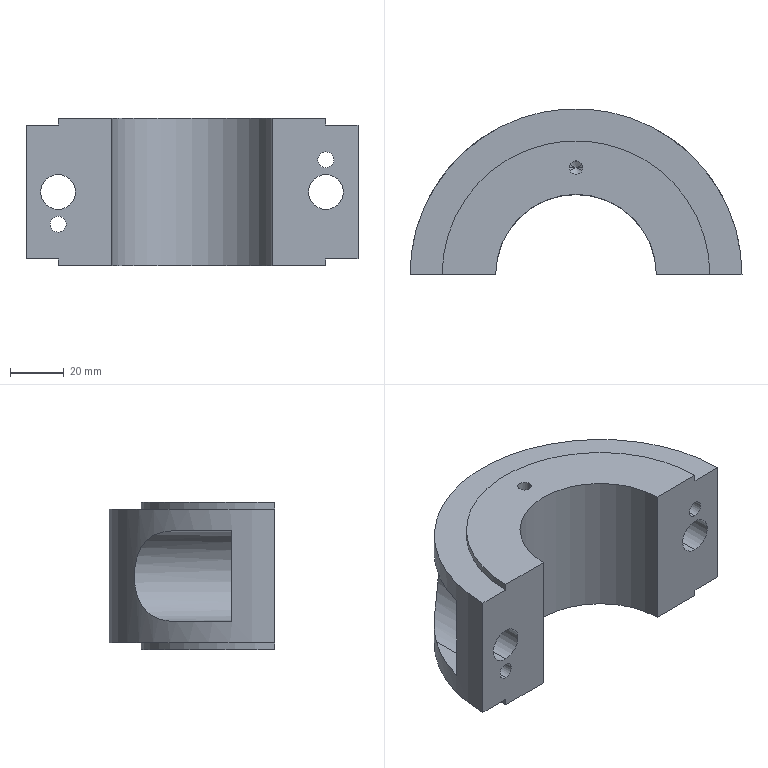Part | SolidWorks | features ICE 3, Extrusion 1, HoleWzd 1 | 1 solid | 30 faces | box 124 x 62 x 55 mm | volume 204402 mm3 | cylinder 16 | plane 12 | cone 2 | commonest cylinder face diameters 6 x4 13 x4 5 x2 34 x2 100 x2 60 x1
STEP:
#1=CARTESIAN_POINT('',(-2.5,40.,10.5));
#2=VERTEX_POINT('',#1);
#3=CARTESIAN_POINT('',(2.5,40.,10.5));
#4=VERTEX_POINT('',#3);
#5=CARTESIAN_POINT('',(0.,40.,10.5));
#6=DIRECTION('',(0.,0.,1.));
#7=DIRECTION('',(1.,0.,0.));
#8=AXIS2_PLACEMENT_3D('',#5,#6,#7);
#9=CIRCLE('',#8,2.5);
#10=EDGE_CURVE('',#2,#4,#9,.T.);
#11=ORIENTED_EDGE('',*,*,#10,.F.);
#12=CARTESIAN_POINT('',(-2.5,40.,27.5));
#13=VERTEX_POINT('',#12);
#14=CARTESIAN_POINT('',(-2.5,40.,27.5));
#15=DIRECTION('',(0.,0.,1.));
#16=VECTOR('',#15,1000.);
#17=LINE('',#14,#16);
#18=EDGE_CURVE('',#2,#13,#17,.T.);
#19=ORIENTED_EDGE('',*,*,#18,.T.);
#20=CARTESIAN_POINT('',(2.5,40.,27.5));
#21=VERTEX_POINT('',#20);
#22=CARTESIAN_POINT('',(0.,40.,27.5));
#23=DIRECTION('',(0.,0.,1.));
#24=DIRECTION('',(1.,0.,0.));
#25=AXIS2_PLACEMENT_3D('',#22,#23,#24);
#26=CIRCLE('',#25,2.5);
#27=EDGE_CURVE('',#13,#21,#26,.T.);
#28=ORIENTED_EDGE('',*,*,#27,.T.);
#29=CARTESIAN_POINT('',(2.5,40.,27.5));
#30=DIRECTION('',(0.,0.,1.));
#31=VECTOR('',#30,1000.);
#32=LINE('',#29,#31);
#33=EDGE_CURVE('',#4,#21,#32,.T.);
#34=ORIENTED_EDGE('',*,*,#33,.F.);
#35=EDGE_LOOP('',(#11,#19,#28,#34));
#36=FACE_OUTER_BOUND('',#35,.T.);
#37=CARTESIAN_POINT('',(0.,40.,27.5));
#38=DIRECTION('',(0.,0.,1.));
#39=DIRECTION('',(1.,0.,0.));
#40=AXIS2_PLACEMENT_3D('',#37,#38,#39);
#41=CYLINDRICAL_SURFACE('',#40,2.5);
#42=ADVANCED_FACE('',(#36),#41,.F.);
#43=CARTESIAN_POINT('',(0.,40.,8.998));
#44=VERTEX_POINT('',#43);
#45=CARTESIAN_POINT('',(2.5,40.,10.5));
#46=DIRECTION('',(0.8572,0.,0.515));
#47=VECTOR('',#46,1000.);
#48=LINE('',#45,#47);
#49=EDGE_CURVE('',#44,#4,#48,.T.);
#50=ORIENTED_EDGE('',*,*,#49,.F.);
#51=CARTESIAN_POINT('',(-2.5,40.,10.5));
#52=DIRECTION('',(-0.8572,0.,0.515));
#53=VECTOR('',#52,1000.);
#54=LINE('',#51,#53);
#55=EDGE_CURVE('',#44,#2,#54,.T.);
#56=ORIENTED_EDGE('',*,*,#55,.T.);
#57=ORIENTED_EDGE('',*,*,#10,.T.);
#58=EDGE_LOOP('',(#50,#56,#57));
#59=FACE_OUTER_BOUND('',#58,.T.);
#60=CARTESIAN_POINT('',(0.,40.,10.5));
#61=DIRECTION('',(0.,0.,1.));
#62=DIRECTION('',(1.,0.,0.));
#63=AXIS2_PLACEMENT_3D('',#60,#61,#62);
#64=CONICAL_SURFACE('',#63,2.5,1.03);
#65=ADVANCED_FACE('',(#59),#64,.F.);
#66=CARTESIAN_POINT('',(50.,0.,-6.5));
#67=VERTEX_POINT('',#66);
#68=CARTESIAN_POINT('',(50.,0.,6.5));
#69=VERTEX_POINT('',#68);
#70=CARTESIAN_POINT('',(50.,0.,0.));
#71=DIRECTION('',(0.,1.,0.));
#72=DIRECTION('',(0.,0.,-1.));
#73=AXIS2_PLACEMENT_3D('',#70,#71,#72);
#74=CIRCLE('',#73,6.5);
#75=EDGE_CURVE('',#67,#69,#74,.T.);
#76=ORIENTED_EDGE('',*,*,#75,.F.);
#77=CARTESIAN_POINT('',(50.,16.,-6.5));
#78=VERTEX_POINT('',#77);
#79=CARTESIAN_POINT('',(50.,0.,-6.5));
#80=DIRECTION('',(0.,1.,0.));
#81=VECTOR('',#80,1000.);
#82=LINE('',#79,#81);
#83=EDGE_CURVE('',#67,#78,#82,.T.);
#84=ORIENTED_EDGE('',*,*,#83,.T.);
#85=CARTESIAN_POINT('',(50.,16.,6.5));
#86=VERTEX_POINT('',#85);
#87=CARTESIAN_POINT('',(50.,16.,0.));
#88=DIRECTION('',(0.,1.,0.));
#89=DIRECTION('',(0.,0.,-1.));
#90=AXIS2_PLACEMENT_3D('',#87,#88,#89);
#91=CIRCLE('',#90,6.5);
#92=EDGE_CURVE('',#78,#86,#91,.T.);
#93=ORIENTED_EDGE('',*,*,#92,.T.);
#94=CARTESIAN_POINT('',(50.,0.,6.5));
#95=DIRECTION('',(0.,1.,0.));
#96=VECTOR('',#95,1000.);
#97=LINE('',#94,#96);
#98=EDGE_CURVE('',#69,#86,#97,.T.);
#99=ORIENTED_EDGE('',*,*,#98,.F.);
#100=EDGE_LOOP('',(#76,#84,#93,#99));
#101=FACE_OUTER_BOUND('',#100,.T.);
#102=CARTESIAN_POINT('',(50.,0.,0.));
#103=DIRECTION('',(0.,1.,0.));
#104=DIRECTION('',(0.,0.,1.));
#105=AXIS2_PLACEMENT_3D('',#102,#103,#104);
#106=CYLINDRICAL_SURFACE('',#105,6.5);
#107=ADVANCED_FACE('',(#101),#106,.F.);
#108=CARTESIAN_POINT('',(50.,0.,9.));
#109=VERTEX_POINT('',#108);
#110=CARTESIAN_POINT('',(50.,0.,15.));
#111=VERTEX_POINT('',#110);
#112=CARTESIAN_POINT('',(50.,0.,12.));
#113=DIRECTION('',(0.,1.,0.));
#114=DIRECTION('',(0.,0.,1.));
#115=AXIS2_PLACEMENT_3D('',#112,#113,#114);
#116=CIRCLE('',#115,3.);
#117=EDGE_CURVE('',#109,#111,#116,.T.);
#118=ORIENTED_EDGE('',*,*,#117,.F.);
#119=CARTESIAN_POINT('',(50.,16.,9.));
#120=VERTEX_POINT('',#119);
#121=CARTESIAN_POINT('',(50.,0.,9.));
#122=DIRECTION('',(0.,1.,0.));
#123=VECTOR('',#122,1000.);
#124=LINE('',#121,#123);
#125=EDGE_CURVE('',#109,#120,#124,.T.);
#126=ORIENTED_EDGE('',*,*,#125,.T.);
#127=CARTESIAN_POINT('',(50.,16.,15.));
#128=VERTEX_POINT('',#127);
#129=CARTESIAN_POINT('',(50.,16.,12.));
#130=DIRECTION('',(0.,1.,0.));
#131=DIRECTION('',(0.,0.,1.));
#132=AXIS2_PLACEMENT_3D('',#129,#130,#131);
#133=CIRCLE('',#132,3.);
#134=EDGE_CURVE('',#120,#128,#133,.T.);
#135=ORIENTED_EDGE('',*,*,#134,.T.);
#136=CARTESIAN_POINT('',(50.,0.,15.));
#137=DIRECTION('',(0.,1.,0.));
#138=VECTOR('',#137,1000.);
#139=LINE('',#136,#138);
#140=EDGE_CURVE('',#111,#128,#139,.T.);
#141=ORIENTED_EDGE('',*,*,#140,.F.);
#142=EDGE_LOOP('',(#118,#126,#135,#141));
#143=FACE_OUTER_BOUND('',#142,.T.);
#144=CARTESIAN_POINT('',(50.,0.,12.));
#145=DIRECTION('',(0.,1.,0.));
#146=DIRECTION('',(0.,0.,1.));
#147=AXIS2_PLACEMENT_3D('',#144,#145,#146);
#148=CYLINDRICAL_SURFACE('',#147,3.);
#149=ADVANCED_FACE('',(#143),#148,.F.);
#150=CARTESIAN_POINT('',(-50.,0.,-15.));
#151=VERTEX_POINT('',#150);
#152=CARTESIAN_POINT('',(-50.,0.,-9.));
#153=VERTEX_POINT('',#152);
#154=CARTESIAN_POINT('',(-50.,0.,-12.));
#155=DIRECTION('',(0.,1.,0.));
#156=DIRECTION('',(0.,0.,1.));
#157=AXIS2_PLACEMENT_3D('',#154,#155,#156);
#158=CIRCLE('',#157,3.);
#159=EDGE_CURVE('',#151,#153,#158,.T.);
#160=ORIENTED_EDGE('',*,*,#159,.F.);
#161=CARTESIAN_POINT('',(-50.,16.,-15.));
#162=VERTEX_POINT('',#161);
#163=CARTESIAN_POINT('',(-50.,0.,-15.));
#164=DIRECTION('',(0.,1.,0.));
#165=VECTOR('',#164,1000.);
#166=LINE('',#163,#165);
#167=EDGE_CURVE('',#151,#162,#166,.T.);
#168=ORIENTED_EDGE('',*,*,#167,.T.);
#169=CARTESIAN_POINT('',(-50.,16.,-9.));
#170=VERTEX_POINT('',#169);
#171=CARTESIAN_POINT('',(-50.,16.,-12.));
#172=DIRECTION('',(0.,1.,0.));
#173=DIRECTION('',(0.,0.,1.));
#174=AXIS2_PLACEMENT_3D('',#171,#172,#173);
#175=CIRCLE('',#174,3.);
#176=EDGE_CURVE('',#162,#170,#175,.T.);
#177=ORIENTED_EDGE('',*,*,#176,.T.);
#178=CARTESIAN_POINT('',(-50.,0.,-9.));
#179=DIRECTION('',(0.,1.,0.));
#180=VECTOR('',#179,1000.);
#181=LINE('',#178,#180);
#182=EDGE_CURVE('',#153,#170,#181,.T.);
#183=ORIENTED_EDGE('',*,*,#182,.F.);
#184=EDGE_LOOP('',(#160,#168,#177,#183));
#185=FACE_OUTER_BOUND('',#184,.T.);
#186=CARTESIAN_POINT('',(-50.,0.,-12.));
#187=DIRECTION('',(0.,1.,0.));
#188=DIRECTION('',(0.,0.,1.));
#189=AXIS2_PLACEMENT_3D('',#186,#187,#188);
#190=CYLINDRICAL_SURFACE('',#189,3.);
#191=ADVANCED_FACE('',(#185),#190,.F.);
#192=CARTESIAN_POINT('',(-50.,0.,-6.5));
#193=VERTEX_POINT('',#192);
#194=CARTESIAN_POINT('',(-50.,0.,6.5));
#195=VERTEX_POINT('',#194);
#196=CARTESIAN_POINT('',(-50.,0.,0.));
#197=DIRECTION('',(0.,1.,0.));
#198=DIRECTION('',(0.,0.,1.));
#199=AXIS2_PLACEMENT_3D('',#196,#197,#198);
#200=CIRCLE('',#199,6.5);
#201=EDGE_CURVE('',#193,#195,#200,.T.);
#202=ORIENTED_EDGE('',*,*,#201,.F.);
#203=CARTESIAN_POINT('',(-50.,16.,-6.5));
#204=VERTEX_POINT('',#203);
#205=CARTESIAN_POINT('',(-50.,0.,-6.5));
#206=DIRECTION('',(0.,1.,0.));
#207=VECTOR('',#206,1000.);
#208=LINE('',#205,#207);
#209=EDGE_CURVE('',#193,#204,#208,.T.);
#210=ORIENTED_EDGE('',*,*,#209,.T.);
#211=CARTESIAN_POINT('',(-50.,16.,6.5));
#212=VERTEX_POINT('',#211);
#213=CARTESIAN_POINT('',(-50.,16.,0.));
#214=DIRECTION('',(0.,1.,0.));
#215=DIRECTION('',(0.,0.,1.));
#216=AXIS2_PLACEMENT_3D('',#213,#214,#215);
#217=CIRCLE('',#216,6.5);
#218=EDGE_CURVE('',#204,#212,#217,.T.);
#219=ORIENTED_EDGE('',*,*,#218,.T.);
#220=CARTESIAN_POINT('',(-50.,0.,6.5));
#221=DIRECTION('',(0.,1.,0.));
#222=VECTOR('',#221,1000.);
#223=LINE('',#220,#222);
#224=EDGE_CURVE('',#195,#212,#223,.T.);
#225=ORIENTED_EDGE('',*,*,#224,.F.);
#226=EDGE_LOOP('',(#202,#210,#219,#225));
#227=FACE_OUTER_BOUND('',#226,.T.);
#228=CARTESIAN_POINT('',(-50.,0.,0.));
#229=DIRECTION('',(0.,1.,0.));
#230=DIRECTION('',(0.,0.,1.));
#231=AXIS2_PLACEMENT_3D('',#228,#229,#230);
#232=CYLINDRICAL_SURFACE('',#231,6.5);
#233=ADVANCED_FACE('',(#227),#232,.F.);
#234=CARTESIAN_POINT('',(-59.9,16.,17.));
#235=VERTEX_POINT('',#234);
#236=CARTESIAN_POINT('',(-50.,36.661,17.));
#237=VERTEX_POINT('',#236);
#238=CARTESIAN_POINT('',(0.,0.,17.));
#239=DIRECTION('',(0.,0.,-1.));
#240=DIRECTION('',(-1.,0.,0.));
#241=AXIS2_PLACEMENT_3D('',#238,#239,#240);
#242=CIRCLE('',#241,62.);
#243=EDGE_CURVE('',#235,#237,#242,.T.);
#244=ORIENTED_EDGE('',*,*,#243,.F.);
#245=CARTESIAN_POINT('',(-59.9,16.,-17.));
#246=VERTEX_POINT('',#245);
#247=CARTESIAN_POINT('',(-59.9,16.,25.));
#248=DIRECTION('',(0.,0.,1.));
#249=VECTOR('',#248,1000.);
#250=LINE('',#247,#249);
#251=EDGE_CURVE('',#246,#235,#250,.T.);
#252=ORIENTED_EDGE('',*,*,#251,.F.);
#253=CARTESIAN_POINT('',(-50.,36.661,-17.));
#254=VERTEX_POINT('',#253);
#255=CARTESIAN_POINT('',(0.,0.,-17.));
#256=DIRECTION('',(0.,0.,1.));
#257=DIRECTION('',(1.,0.,0.));
#258=AXIS2_PLACEMENT_3D('',#255,#256,#257);
#259=CIRCLE('',#258,62.);
#260=EDGE_CURVE('',#254,#246,#259,.T.);
#261=ORIENTED_EDGE('',*,*,#260,.F.);
#262=CARTESIAN_POINT('',(-50.,36.661,17.));
#263=CARTESIAN_POINT('',(-49.604,37.2,17.));
#264=CARTESIAN_POINT('',(-49.2,37.734,16.986));
#265=CARTESIAN_POINT('',(-48.372,38.789,16.927));
#266=CARTESIAN_POINT('',(-47.948,39.312,16.881));
#267=CARTESIAN_POINT('',(-46.654,40.856,16.69));
#268=CARTESIAN_POINT('',(-45.769,41.843,16.492));
#269=CARTESIAN_POINT('',(-43.968,43.732,15.922));
#270=CARTESIAN_POINT('',(-43.051,44.634,15.55));
#271=CARTESIAN_POINT('',(-41.662,45.921,14.824));
#272=CARTESIAN_POINT('',(-41.199,46.335,14.555));
#273=CARTESIAN_POINT('',(-40.29,47.128,13.965));
#274=CARTESIAN_POINT('',(-39.842,47.507,13.643));
#275=CARTESIAN_POINT('',(-38.961,48.232,12.941));
#276=CARTESIAN_POINT('',(-38.529,48.578,12.56));
#277=CARTESIAN_POINT('',(-37.897,49.071,11.941));
#278=CARTESIAN_POINT('',(-37.688,49.231,11.726));
#279=CARTESIAN_POINT('',(-37.281,49.54,11.283));
#280=CARTESIAN_POINT('',(-37.082,49.689,11.055));
#281=CARTESIAN_POINT('',(-36.117,50.404,9.885));
#282=CARTESIAN_POINT('',(-35.429,50.885,8.85));
#283=CARTESIAN_POINT('',(-34.555,51.479,7.132));
#284=CARTESIAN_POINT('',(-34.289,51.656,6.527));
#285=CARTESIAN_POINT('',(-33.832,51.956,5.295));
#286=CARTESIAN_POINT('',(-33.639,52.081,4.666));
#287=CARTESIAN_POINT('',(-33.326,52.282,3.381));
#288=CARTESIAN_POINT('',(-33.206,52.358,2.725));
#289=CARTESIAN_POINT('',(-33.084,52.435,1.72));
#290=CARTESIAN_POINT('',(-33.053,52.455,1.381));
#291=CARTESIAN_POINT('',(-33.011,52.481,0.7054));
#292=CARTESIAN_POINT('',(-33.001,52.488,0.3685));
#293=CARTESIAN_POINT('',(-32.999,52.489,-0.6399));
#294=CARTESIAN_POINT('',(-33.037,52.465,-1.309));
#295=CARTESIAN_POINT('',(-33.154,52.391,-2.308));
#296=CARTESIAN_POINT('',(-33.203,52.36,-2.641));
#297=CARTESIAN_POINT('',(-33.321,52.285,-3.304));
#298=CARTESIAN_POINT('',(-33.39,52.241,-3.635));
#299=CARTESIAN_POINT('',(-33.78,51.991,-5.263));
#300=CARTESIAN_POINT('',(-34.235,51.696,-6.492));
#301=CARTESIAN_POINT('',(-34.965,51.2,-7.941));
#302=CARTESIAN_POINT('',(-35.119,51.095,-8.226));
#303=CARTESIAN_POINT('',(-35.439,50.874,-8.779));
#304=CARTESIAN_POINT('',(-35.605,50.758,-9.048));
#305=CARTESIAN_POINT('',(-36.12,50.394,-9.836));
#306=CARTESIAN_POINT('',(-36.487,50.129,-10.333));
#307=CARTESIAN_POINT('',(-37.262,49.555,-11.275));
#308=CARTESIAN_POINT('',(-37.673,49.244,-11.722));
#309=CARTESIAN_POINT('',(-38.517,48.587,-12.549));
#310=CARTESIAN_POINT('',(-38.95,48.241,-12.931));
#311=CARTESIAN_POINT('',(-39.834,47.514,-13.637));
#312=CARTESIAN_POINT('',(-40.285,47.133,-13.961));
#313=CARTESIAN_POINT('',(-41.2,46.335,-14.556));
#314=CARTESIAN_POINT('',(-41.665,45.918,-14.826));
#315=CARTESIAN_POINT('',(-43.048,44.637,-15.548));
#316=CARTESIAN_POINT('',(-43.964,43.736,-15.921));
#317=CARTESIAN_POINT('',(-45.319,42.316,-16.35));
#318=CARTESIAN_POINT('',(-45.767,41.831,-16.471));
#319=CARTESIAN_POINT('',(-46.655,40.838,-16.674));
#320=CARTESIAN_POINT('',(-47.096,40.329,-16.756));
#321=CARTESIAN_POINT('',(-48.387,38.788,-16.946));
#322=CARTESIAN_POINT('',(-49.211,37.737,-17.));
#323=CARTESIAN_POINT('',(-50.,36.661,-17.));
#324=B_SPLINE_CURVE_WITH_KNOTS('',3,(#262,#263,#264,#265,#266,#267,#268,#269,#270,#271,#272,#273,#274,#275,#276,#277,#278,#279,#280,#281,#282,#283,#284,#285,#286,#287,#288,#289,#290,#291,#292,#293,#294,#295,#296,#297,#298,#299,#300,#301,#302,#303,#304,#305,#306,#307,#308,#309,#310,#311,#312,#313,#314,#315,#316,#317,#318,#319,#320,#321,#322,#323),.UNSPECIFIED.,.F.,.F.,(4,2,2,2,2,2,2,2,2,2,2,2,2,2,2,2,2,2,2,2,2,2,2,2,2,2,2,2,2,2,4),(0.03941,0.04141,0.04341,0.0474,0.0514,0.05339,0.05539,0.05739,0.05839,0.05938,0.06338,0.06538,0.06737,0.06937,0.07037,0.07137,0.07336,0.07436,0.07536,0.07935,0.08035,0.08135,0.08335,0.08534,0.08734,0.08934,0.09134,0.09533,0.09733,0.09932,0.1033),.UNSPECIFIED.);
#325=EDGE_CURVE('',#237,#254,#324,.T.);
#326=ORIENTED_EDGE('',*,*,#325,.F.);
#327=EDGE_LOOP('',(#244,#252,#261,#326));
#328=FACE_BOUND('',#327,.T.);
#329=CARTESIAN_POINT('',(62.,0.,-25.));
#330=VERTEX_POINT('',#329);
#331=CARTESIAN_POINT('',(-62.,0.,-25.));
#332=VERTEX_POINT('',#331);
#333=CARTESIAN_POINT('',(0.,0.,-25.));
#334=DIRECTION('',(0.,0.,1.));
#335=DIRECTION('',(1.,0.,0.));
#336=AXIS2_PLACEMENT_3D('',#333,#334,#335);
#337=CIRCLE('',#336,62.);
#338=EDGE_CURVE('',#330,#332,#337,.T.);
#339=ORIENTED_EDGE('',*,*,#338,.T.);
#340=CARTESIAN_POINT('',(-62.,0.,25.));
#341=VERTEX_POINT('',#340);
#342=CARTESIAN_POINT('',(-62.,0.,25.));
#343=DIRECTION('',(0.,0.,-1.));
#344=VECTOR('',#343,1000.);
#345=LINE('',#342,#344);
#346=EDGE_CURVE('',#341,#332,#345,.T.);
#347=ORIENTED_EDGE('',*,*,#346,.F.);
#348=CARTESIAN_POINT('',(62.,0.,25.));
#349=VERTEX_POINT('',#348);
#350=CARTESIAN_POINT('',(0.,0.,25.));
#351=DIRECTION('',(0.,0.,1.));
#352=DIRECTION('',(1.,0.,0.));
#353=AXIS2_PLACEMENT_3D('',#350,#351,#352);
#354=CIRCLE('',#353,62.);
#355=EDGE_CURVE('',#349,#341,#354,.T.);
#356=ORIENTED_EDGE('',*,*,#355,.F.);
#357=CARTESIAN_POINT('',(62.,0.,25.));
#358=DIRECTION('',(0.,0.,-1.));
#359=VECTOR('',#358,1000.);
#360=LINE('',#357,#359);
#361=EDGE_CURVE('',#349,#330,#360,.T.);
#362=ORIENTED_EDGE('',*,*,#361,.T.);
#363=EDGE_LOOP('',(#339,#347,#356,#362));
#364=FACE_OUTER_BOUND('',#363,.T.);
#365=CARTESIAN_POINT('',(50.,36.661,-17.));
#366=VERTEX_POINT('',#365);
#367=CARTESIAN_POINT('',(50.,36.661,17.));
#368=VERTEX_POINT('',#367);
#369=CARTESIAN_POINT('',(50.,36.661,-17.));
#370=CARTESIAN_POINT('',(49.209,37.739,-17.));
#371=CARTESIAN_POINT('',(48.383,38.793,-16.945));
#372=CARTESIAN_POINT('',(47.091,40.335,-16.755));
#373=CARTESIAN_POINT('',(46.651,40.843,-16.673));
#374=CARTESIAN_POINT('',(45.765,41.833,-16.47));
#375=CARTESIAN_POINT('',(45.318,42.316,-16.349));
#376=CARTESIAN_POINT('',(43.966,43.734,-15.921));
#377=CARTESIAN_POINT('',(43.051,44.634,-15.55));
#378=CARTESIAN_POINT('',(41.667,45.916,-14.827));
#379=CARTESIAN_POINT('',(41.202,46.333,-14.557));
#380=CARTESIAN_POINT('',(40.291,47.128,-13.965));
#381=CARTESIAN_POINT('',(39.841,47.508,-13.643));
#382=CARTESIAN_POINT('',(38.961,48.232,-12.941));
#383=CARTESIAN_POINT('',(38.53,48.577,-12.561));
#384=CARTESIAN_POINT('',(37.689,49.232,-11.739));
#385=CARTESIAN_POINT('',(37.278,49.544,-11.293));
#386=CARTESIAN_POINT('',(36.114,50.405,-9.883));
#387=CARTESIAN_POINT('',(35.426,50.887,-8.846));
#388=CARTESIAN_POINT('',(34.701,51.38,-7.419));
#389=CARTESIAN_POINT('',(34.563,51.473,-7.127));
#390=CARTESIAN_POINT('',(34.3,51.648,-6.529));
#391=CARTESIAN_POINT('',(34.176,51.73,-6.222));
#392=CARTESIAN_POINT('',(33.832,51.956,-5.294));
#393=CARTESIAN_POINT('',(33.639,52.081,-4.664));
#394=CARTESIAN_POINT('',(33.326,52.282,-3.378));
#395=CARTESIAN_POINT('',(33.206,52.358,-2.724));
#396=CARTESIAN_POINT('',(33.044,52.461,-1.389));
#397=CARTESIAN_POINT('',(33.001,52.487,-0.7059));
#398=CARTESIAN_POINT('',(32.999,52.489,0.6414));
#399=CARTESIAN_POINT('',(33.037,52.465,1.311));
#400=CARTESIAN_POINT('',(33.154,52.391,2.309));
#401=CARTESIAN_POINT('',(33.203,52.36,2.64));
#402=CARTESIAN_POINT('',(33.32,52.285,3.301));
#403=CARTESIAN_POINT('',(33.389,52.242,3.632));
#404=CARTESIAN_POINT('',(33.78,51.991,5.264));
#405=CARTESIAN_POINT('',(34.235,51.696,6.493));
#406=CARTESIAN_POINT('',(34.963,51.202,7.937));
#407=CARTESIAN_POINT('',(35.117,51.096,8.223));
#408=CARTESIAN_POINT('',(35.438,50.874,8.777));
#409=CARTESIAN_POINT('',(35.604,50.758,9.047));
#410=CARTESIAN_POINT('',(36.12,50.394,9.835));
#411=CARTESIAN_POINT('',(36.487,50.129,10.333));
#412=CARTESIAN_POINT('',(37.067,49.7,11.038));
#413=CARTESIAN_POINT('',(37.266,49.551,11.267));
#414=CARTESIAN_POINT('',(37.673,49.242,11.71));
#415=CARTESIAN_POINT('',(37.882,49.082,11.926));
#416=CARTESIAN_POINT('',(38.516,48.588,12.548));
#417=CARTESIAN_POINT('',(38.949,48.242,12.93));
#418=CARTESIAN_POINT('',(39.833,47.515,13.636));
#419=CARTESIAN_POINT('',(40.283,47.134,13.96));
#420=CARTESIAN_POINT('',(41.197,46.338,14.554));
#421=CARTESIAN_POINT('',(41.662,45.92,14.824));
#422=CARTESIAN_POINT('',(43.048,44.637,15.548));
#423=CARTESIAN_POINT('',(43.965,43.736,15.921));
#424=CARTESIAN_POINT('',(45.318,42.317,16.349));
#425=CARTESIAN_POINT('',(45.765,41.833,16.47));
#426=CARTESIAN_POINT('',(46.652,40.842,16.673));
#427=CARTESIAN_POINT('',(47.092,40.334,16.755));
#428=CARTESIAN_POINT('',(48.386,38.79,16.946));
#429=CARTESIAN_POINT('',(49.211,37.737,17.));
#430=CARTESIAN_POINT('',(50.,36.661,17.));
#431=B_SPLINE_CURVE_WITH_KNOTS('',3,(#369,#370,#371,#372,#373,#374,#375,#376,#377,#378,#379,#380,#381,#382,#383,#384,#385,#386,#387,#388,#389,#390,#391,#392,#393,#394,#395,#396,#397,#398,#399,#400,#401,#402,#403,#404,#405,#406,#407,#408,#409,#410,#411,#412,#413,#414,#415,#416,#417,#418,#419,#420,#421,#422,#423,#424,#425,#426,#427,#428,#429,#430),.UNSPECIFIED.,.F.,.F.,(4,2,2,2,2,2,2,2,2,2,2,2,2,2,2,2,2,2,2,2,2,2,2,2,2,2,2,2,2,2,4),(0.05777,0.06177,0.06376,0.06576,0.06975,0.07175,0.07374,0.07574,0.07773,0.08172,0.08272,0.08372,0.08572,0.08771,0.08971,0.0917,0.0927,0.0937,0.09769,0.09869,0.09969,0.1017,0.1027,0.1037,0.1057,0.1077,0.1097,0.1137,0.1157,0.1176,0.1216),.UNSPECIFIED.);
#432=EDGE_CURVE('',#366,#368,#431,.T.);
#433=ORIENTED_EDGE('',*,*,#432,.F.);
#434=CARTESIAN_POINT('',(59.9,16.,-17.));
#435=VERTEX_POINT('',#434);
#436=CARTESIAN_POINT('',(0.,0.,-17.));
#437=DIRECTION('',(0.,0.,1.));
#438=DIRECTION('',(1.,0.,0.));
#439=AXIS2_PLACEMENT_3D('',#436,#437,#438);
#440=CIRCLE('',#439,62.);
#441=EDGE_CURVE('',#435,#366,#440,.T.);
#442=ORIENTED_EDGE('',*,*,#441,.F.);
#443=CARTESIAN_POINT('',(59.9,16.,17.));
#444=VERTEX_POINT('',#443);
#445=CARTESIAN_POINT('',(59.9,16.,25.));
#446=DIRECTION('',(0.,0.,1.));
#447=VECTOR('',#446,1000.);
#448=LINE('',#445,#447);
#449=EDGE_CURVE('',#435,#444,#448,.T.);
#450=ORIENTED_EDGE('',*,*,#449,.T.);
#451=CARTESIAN_POINT('',(0.,0.,17.));
#452=DIRECTION('',(0.,0.,-1.));
#453=DIRECTION('',(-1.,0.,0.));
#454=AXIS2_PLACEMENT_3D('',#451,#452,#453);
#455=CIRCLE('',#454,62.);
#456=EDGE_CURVE('',#368,#444,#455,.T.);
#457=ORIENTED_EDGE('',*,*,#456,.F.);
#458=EDGE_LOOP('',(#433,#442,#450,#457));
#459=FACE_BOUND('',#458,.T.);
#460=CARTESIAN_POINT('',(0.,0.,25.));
#461=DIRECTION('',(0.,0.,-1.));
#462=DIRECTION('',(-1.,0.,0.));
#463=AXIS2_PLACEMENT_3D('',#460,#461,#462);
#464=CYLINDRICAL_SURFACE('',#463,62.);
#465=ADVANCED_FACE('',(#328,#364,#459),#464,.T.);
#466=CARTESIAN_POINT('',(-50.,0.,25.));
#467=VERTEX_POINT('',#466);
#468=CARTESIAN_POINT('',(-62.,0.,25.));
#469=DIRECTION('',(1.,0.,0.));
#470=VECTOR('',#469,1000.);
#471=LINE('',#468,#470);
#472=EDGE_CURVE('',#341,#467,#471,.T.);
#473=ORIENTED_EDGE('',*,*,#472,.T.);
#474=CARTESIAN_POINT('',(50.,0.,25.));
#475=VERTEX_POINT('',#474);
#476=CARTESIAN_POINT('',(0.,0.,25.));
#477=DIRECTION('',(0.,0.,-1.));
#478=DIRECTION('',(1.,0.,0.));
#479=AXIS2_PLACEMENT_3D('',#476,#477,#478);
#480=CIRCLE('',#479,50.);
#481=EDGE_CURVE('',#467,#475,#480,.T.);
#482=ORIENTED_EDGE('',*,*,#481,.T.);
#483=CARTESIAN_POINT('',(30.,0.,25.));
#484=DIRECTION('',(1.,0.,0.));
#485=VECTOR('',#484,1000.);
#486=LINE('',#483,#485);
#487=EDGE_CURVE('',#475,#349,#486,.T.);
#488=ORIENTED_EDGE('',*,*,#487,.T.);
#489=ORIENTED_EDGE('',*,*,#355,.T.);
#490=EDGE_LOOP('',(#473,#482,#488,#489));
#491=FACE_OUTER_BOUND('',#490,.T.);
#492=CARTESIAN_POINT('',(0.,0.,25.));
#493=DIRECTION('',(0.,0.,1.));
#494=DIRECTION('',(1.,0.,0.));
#495=AXIS2_PLACEMENT_3D('',#492,#493,#494);
#496=PLANE('',#495);
#497=ADVANCED_FACE('',(#491),#496,.T.);
#498=CARTESIAN_POINT('',(-50.,0.,-25.));
#499=VERTEX_POINT('',#498);
#500=CARTESIAN_POINT('',(50.,0.,-25.));
#501=VERTEX_POINT('',#500);
#502=CARTESIAN_POINT('',(0.,0.,-25.));
#503=DIRECTION('',(0.,0.,-1.));
#504=DIRECTION('',(1.,0.,0.));
#505=AXIS2_PLACEMENT_3D('',#502,#503,#504);
#506=CIRCLE('',#505,50.);
#507=EDGE_CURVE('',#499,#501,#506,.T.);
#508=ORIENTED_EDGE('',*,*,#507,.F.);
#509=CARTESIAN_POINT('',(-62.,0.,-25.));
#510=DIRECTION('',(1.,0.,0.));
#511=VECTOR('',#510,1000.);
#512=LINE('',#509,#511);
#513=EDGE_CURVE('',#332,#499,#512,.T.);
#514=ORIENTED_EDGE('',*,*,#513,.F.);
#515=ORIENTED_EDGE('',*,*,#338,.F.);
#516=CARTESIAN_POINT('',(30.,0.,-25.));
#517=DIRECTION('',(1.,0.,0.));
#518=VECTOR('',#517,1000.);
#519=LINE('',#516,#518);
#520=EDGE_CURVE('',#501,#330,#519,.T.);
#521=ORIENTED_EDGE('',*,*,#520,.F.);
#522=EDGE_LOOP('',(#508,#514,#515,#521));
#523=FACE_OUTER_BOUND('',#522,.T.);
#524=CARTESIAN_POINT('',(0.,0.,-25.));
#525=DIRECTION('',(0.,0.,1.));
#526=DIRECTION('',(1.,0.,0.));
#527=AXIS2_PLACEMENT_3D('',#524,#525,#526);
#528=PLANE('',#527);
#529=ADVANCED_FACE('',(#523),#528,.F.);
#530=CARTESIAN_POINT('',(-50.,0.,-12.));
#531=DIRECTION('',(0.,1.,0.));
#532=DIRECTION('',(0.,0.,1.));
#533=AXIS2_PLACEMENT_3D('',#530,#531,#532);
#534=CIRCLE('',#533,3.);
#535=EDGE_CURVE('',#153,#151,#534,.T.);
#536=ORIENTED_EDGE('',*,*,#535,.T.);
#537=ORIENTED_EDGE('',*,*,#159,.T.);
#538=EDGE_LOOP('',(#536,#537));
#539=FACE_BOUND('',#538,.T.);
#540=CARTESIAN_POINT('',(-50.,0.,0.));
#541=DIRECTION('',(0.,1.,0.));
#542=DIRECTION('',(0.,0.,1.));
#543=AXIS2_PLACEMENT_3D('',#540,#541,#542);
#544=CIRCLE('',#543,6.5);
#545=EDGE_CURVE('',#195,#193,#544,.T.);
#546=ORIENTED_EDGE('',*,*,#545,.T.);
#547=ORIENTED_EDGE('',*,*,#201,.T.);
#548=EDGE_LOOP('',(#546,#547));
#549=FACE_BOUND('',#548,.T.);
#550=CARTESIAN_POINT('',(-30.,0.,27.5));
#551=VERTEX_POINT('',#550);
#552=CARTESIAN_POINT('',(-30.,0.,-27.5));
#553=VERTEX_POINT('',#552);
#554=CARTESIAN_POINT('',(-30.,0.,25.));
#555=DIRECTION('',(0.,0.,-1.));
#556=VECTOR('',#555,1000.);
#557=LINE('',#554,#556);
#558=EDGE_CURVE('',#551,#553,#557,.T.);
#559=ORIENTED_EDGE('',*,*,#558,.F.);
#560=CARTESIAN_POINT('',(-50.,0.,27.5));
#561=VERTEX_POINT('',#560);
#562=CARTESIAN_POINT('',(-50.,0.,27.5));
#563=DIRECTION('',(1.,0.,0.));
#564=VECTOR('',#563,1000.);
#565=LINE('',#562,#564);
#566=EDGE_CURVE('',#561,#551,#565,.T.);
#567=ORIENTED_EDGE('',*,*,#566,.F.);
#568=CARTESIAN_POINT('',(-50.,0.,27.5));
#569=DIRECTION('',(0.,0.,-1.));
#570=VECTOR('',#569,1000.);
#571=LINE('',#568,#570);
#572=EDGE_CURVE('',#561,#467,#571,.T.);
#573=ORIENTED_EDGE('',*,*,#572,.T.);
#574=ORIENTED_EDGE('',*,*,#472,.F.);
#575=ORIENTED_EDGE('',*,*,#346,.T.);
#576=ORIENTED_EDGE('',*,*,#513,.T.);
#577=CARTESIAN_POINT('',(-50.,0.,-27.5));
#578=VERTEX_POINT('',#577);
#579=CARTESIAN_POINT('',(-50.,0.,27.5));
#580=DIRECTION('',(0.,0.,-1.));
#581=VECTOR('',#580,1000.);
#582=LINE('',#579,#581);
#583=EDGE_CURVE('',#499,#578,#582,.T.);
#584=ORIENTED_EDGE('',*,*,#583,.T.);
#585=CARTESIAN_POINT('',(-50.,0.,-27.5));
#586=DIRECTION('',(1.,0.,0.));
#587=VECTOR('',#586,1000.);
#588=LINE('',#585,#587);
#589=EDGE_CURVE('',#578,#553,#588,.T.);
#590=ORIENTED_EDGE('',*,*,#589,.T.);
#591=EDGE_LOOP('',(#559,#567,#573,#574,#575,#576,#584,#590));
#592=FACE_OUTER_BOUND('',#591,.T.);
#593=CARTESIAN_POINT('',(-62.,0.,25.));
#594=DIRECTION('',(0.,1.,0.));
#595=DIRECTION('',(0.,0.,1.));
#596=AXIS2_PLACEMENT_3D('',#593,#594,#595);
#597=PLANE('',#596);
#598=ADVANCED_FACE('',(#539,#549,#592),#597,.F.);
#599=ORIENTED_EDGE('',*,*,#558,.T.);
#600=CARTESIAN_POINT('',(30.,0.,-27.5));
#601=VERTEX_POINT('',#600);
#602=CARTESIAN_POINT('',(0.,0.,-27.5));
#603=DIRECTION('',(0.,0.,-1.));
#604=DIRECTION('',(1.,0.,0.));
#605=AXIS2_PLACEMENT_3D('',#602,#603,#604);
#606=CIRCLE('',#605,30.);
#607=EDGE_CURVE('',#553,#601,#606,.T.);
#608=ORIENTED_EDGE('',*,*,#607,.T.);
#609=CARTESIAN_POINT('',(30.,0.,27.5));
#610=VERTEX_POINT('',#609);
#611=CARTESIAN_POINT('',(30.,0.,25.));
#612=DIRECTION('',(0.,0.,-1.));
#613=VECTOR('',#612,1000.);
#614=LINE('',#611,#613);
#615=EDGE_CURVE('',#610,#601,#614,.T.);
#616=ORIENTED_EDGE('',*,*,#615,.F.);
#617=CARTESIAN_POINT('',(0.,0.,27.5));
#618=DIRECTION('',(0.,0.,-1.));
#619=DIRECTION('',(1.,0.,0.));
#620=AXIS2_PLACEMENT_3D('',#617,#618,#619);
#621=CIRCLE('',#620,30.);
#622=EDGE_CURVE('',#551,#610,#621,.T.);
#623=ORIENTED_EDGE('',*,*,#622,.F.);
#624=EDGE_LOOP('',(#599,#608,#616,#623));
#625=FACE_OUTER_BOUND('',#624,.T.);
#626=CARTESIAN_POINT('',(0.,0.,25.));
#627=DIRECTION('',(0.,0.,-1.));
#628=DIRECTION('',(-1.,0.,0.));
#629=AXIS2_PLACEMENT_3D('',#626,#627,#628);
#630=CYLINDRICAL_SURFACE('',#629,30.);
#631=ADVANCED_FACE('',(#625),#630,.F.);
#632=CARTESIAN_POINT('',(50.,0.,0.));
#633=DIRECTION('',(0.,1.,0.));
#634=DIRECTION('',(0.,0.,-1.));
#635=AXIS2_PLACEMENT_3D('',#632,#633,#634);
#636=CIRCLE('',#635,6.5);
#637=EDGE_CURVE('',#69,#67,#636,.T.);
#638=ORIENTED_EDGE('',*,*,#637,.T.);
#639=ORIENTED_EDGE('',*,*,#75,.T.);
#640=EDGE_LOOP('',(#638,#639));
#641=FACE_BOUND('',#640,.T.);
#642=CARTESIAN_POINT('',(50.,0.,12.));
#643=DIRECTION('',(0.,1.,0.));
#644=DIRECTION('',(0.,0.,1.));
#645=AXIS2_PLACEMENT_3D('',#642,#643,#644);
#646=CIRCLE('',#645,3.);
#647=EDGE_CURVE('',#111,#109,#646,.T.);
#648=ORIENTED_EDGE('',*,*,#647,.T.);
#649=ORIENTED_EDGE('',*,*,#117,.T.);
#650=EDGE_LOOP('',(#648,#649));
#651=FACE_BOUND('',#650,.T.);
#652=ORIENTED_EDGE('',*,*,#615,.T.);
#653=CARTESIAN_POINT('',(50.,0.,-27.5));
#654=VERTEX_POINT('',#653);
#655=CARTESIAN_POINT('',(30.,0.,-27.5));
#656=DIRECTION('',(1.,0.,0.));
#657=VECTOR('',#656,1000.);
#658=LINE('',#655,#657);
#659=EDGE_CURVE('',#601,#654,#658,.T.);
#660=ORIENTED_EDGE('',*,*,#659,.T.);
#661=CARTESIAN_POINT('',(50.,0.,27.5));
#662=DIRECTION('',(0.,0.,-1.));
#663=VECTOR('',#662,1000.);
#664=LINE('',#661,#663);
#665=EDGE_CURVE('',#501,#654,#664,.T.);
#666=ORIENTED_EDGE('',*,*,#665,.F.);
#667=ORIENTED_EDGE('',*,*,#520,.T.);
#668=ORIENTED_EDGE('',*,*,#361,.F.);
#669=ORIENTED_EDGE('',*,*,#487,.F.);
#670=CARTESIAN_POINT('',(50.,0.,27.5));
#671=VERTEX_POINT('',#670);
#672=CARTESIAN_POINT('',(50.,0.,27.5));
#673=DIRECTION('',(0.,0.,-1.));
#674=VECTOR('',#673,1000.);
#675=LINE('',#672,#674);
#676=EDGE_CURVE('',#671,#475,#675,.T.);
#677=ORIENTED_EDGE('',*,*,#676,.F.);
#678=CARTESIAN_POINT('',(30.,0.,27.5));
#679=DIRECTION('',(1.,0.,0.));
#680=VECTOR('',#679,1000.);
#681=LINE('',#678,#680);
#682=EDGE_CURVE('',#610,#671,#681,.T.);
#683=ORIENTED_EDGE('',*,*,#682,.F.);
#684=EDGE_LOOP('',(#652,#660,#666,#667,#668,#669,#677,#683));
#685=FACE_OUTER_BOUND('',#684,.T.);
#686=CARTESIAN_POINT('',(30.,0.,25.));
#687=DIRECTION('',(0.,1.,0.));
#688=DIRECTION('',(0.,0.,1.));
#689=AXIS2_PLACEMENT_3D('',#686,#687,#688);
#690=PLANE('',#689);
#691=ADVANCED_FACE('',(#641,#651,#685),#690,.F.);
#692=CARTESIAN_POINT('',(0.,0.,-27.5));
#693=DIRECTION('',(0.,0.,1.));
#694=DIRECTION('',(1.,0.,0.));
#695=AXIS2_PLACEMENT_3D('',#692,#693,#694);
#696=CIRCLE('',#695,50.);
#697=EDGE_CURVE('',#654,#578,#696,.T.);
#698=ORIENTED_EDGE('',*,*,#697,.F.);
#699=ORIENTED_EDGE('',*,*,#659,.F.);
#700=ORIENTED_EDGE('',*,*,#607,.F.);
#701=ORIENTED_EDGE('',*,*,#589,.F.);
#702=EDGE_LOOP('',(#698,#699,#700,#701));
#703=FACE_OUTER_BOUND('',#702,.T.);
#704=CARTESIAN_POINT('',(0.,0.,-27.5));
#705=DIRECTION('',(0.,0.,1.));
#706=DIRECTION('',(1.,0.,0.));
#707=AXIS2_PLACEMENT_3D('',#704,#705,#706);
#708=PLANE('',#707);
#709=ADVANCED_FACE('',(#703),#708,.F.);
#710=ORIENTED_EDGE('',*,*,#583,.F.);
#711=ORIENTED_EDGE('',*,*,#507,.T.);
#712=ORIENTED_EDGE('',*,*,#665,.T.);
#713=ORIENTED_EDGE('',*,*,#697,.T.);
#714=EDGE_LOOP('',(#710,#711,#712,#713));
#715=FACE_OUTER_BOUND('',#714,.T.);
#716=CARTESIAN_POINT('',(0.,0.,27.5));
#717=DIRECTION('',(0.,0.,-1.));
#718=DIRECTION('',(-1.,0.,0.));
#719=AXIS2_PLACEMENT_3D('',#716,#717,#718);
#720=CYLINDRICAL_SURFACE('',#719,50.);
#721=ADVANCED_FACE('',(#715),#720,.T.);
#722=ORIENTED_EDGE('',*,*,#481,.F.);
#723=ORIENTED_EDGE('',*,*,#572,.F.);
#724=CARTESIAN_POINT('',(0.,0.,27.5));
#725=DIRECTION('',(0.,0.,1.));
#726=DIRECTION('',(1.,0.,0.));
#727=AXIS2_PLACEMENT_3D('',#724,#725,#726);
#728=CIRCLE('',#727,50.);
#729=EDGE_CURVE('',#671,#561,#728,.T.);
#730=ORIENTED_EDGE('',*,*,#729,.F.);
#731=ORIENTED_EDGE('',*,*,#676,.T.);
#732=EDGE_LOOP('',(#722,#723,#730,#731));
#733=FACE_OUTER_BOUND('',#732,.T.);
#734=CARTESIAN_POINT('',(0.,0.,27.5));
#735=DIRECTION('',(0.,0.,-1.));
#736=DIRECTION('',(-1.,0.,0.));
#737=AXIS2_PLACEMENT_3D('',#734,#735,#736);
#738=CYLINDRICAL_SURFACE('',#737,50.);
#739=ADVANCED_FACE('',(#733),#738,.T.);
#740=CARTESIAN_POINT('',(0.,40.,27.5));
#741=DIRECTION('',(0.,0.,1.));
#742=DIRECTION('',(1.,0.,0.));
#743=AXIS2_PLACEMENT_3D('',#740,#741,#742);
#744=CIRCLE('',#743,2.5);
#745=EDGE_CURVE('',#21,#13,#744,.T.);
#746=ORIENTED_EDGE('',*,*,#745,.F.);
#747=ORIENTED_EDGE('',*,*,#27,.F.);
#748=EDGE_LOOP('',(#746,#747));
#749=FACE_BOUND('',#748,.T.);
#750=ORIENTED_EDGE('',*,*,#729,.T.);
#751=ORIENTED_EDGE('',*,*,#566,.T.);
#752=ORIENTED_EDGE('',*,*,#622,.T.);
#753=ORIENTED_EDGE('',*,*,#682,.T.);
#754=EDGE_LOOP('',(#750,#751,#752,#753));
#755=FACE_OUTER_BOUND('',#754,.T.);
#756=CARTESIAN_POINT('',(0.,0.,27.5));
#757=DIRECTION('',(0.,0.,1.));
#758=DIRECTION('',(1.,0.,0.));
#759=AXIS2_PLACEMENT_3D('',#756,#757,#758);
#760=PLANE('',#759);
#761=ADVANCED_FACE('',(#749,#755),#760,.T.);
#762=ORIENTED_EDGE('',*,*,#243,.T.);
#763=CARTESIAN_POINT('',(-50.,16.,17.));
#764=VERTEX_POINT('',#763);
#765=CARTESIAN_POINT('',(-50.,62.,17.));
#766=DIRECTION('',(0.,-1.,0.));
#767=VECTOR('',#766,1000.);
#768=LINE('',#765,#767);
#769=EDGE_CURVE('',#237,#764,#768,.T.);
#770=ORIENTED_EDGE('',*,*,#769,.T.);
#771=CARTESIAN_POINT('',(-75.,16.,17.));
#772=DIRECTION('',(1.,0.,0.));
#773=VECTOR('',#772,1000.);
#774=LINE('',#771,#773);
#775=EDGE_CURVE('',#235,#764,#774,.T.);
#776=ORIENTED_EDGE('',*,*,#775,.F.);
#777=EDGE_LOOP('',(#762,#770,#776));
#778=FACE_OUTER_BOUND('',#777,.T.);
#779=CARTESIAN_POINT('',(-75.,62.,17.));
#780=DIRECTION('',(0.,0.,-1.));
#781=DIRECTION('',(-1.,0.,0.));
#782=AXIS2_PLACEMENT_3D('',#779,#780,#781);
#783=PLANE('',#782);
#784=ADVANCED_FACE('',(#778),#783,.T.);
#785=ORIENTED_EDGE('',*,*,#325,.T.);
#786=CARTESIAN_POINT('',(-50.,16.,-17.));
#787=VERTEX_POINT('',#786);
#788=CARTESIAN_POINT('',(-50.,62.,-17.));
#789=DIRECTION('',(0.,-1.,0.));
#790=VECTOR('',#789,1000.);
#791=LINE('',#788,#790);
#792=EDGE_CURVE('',#254,#787,#791,.T.);
#793=ORIENTED_EDGE('',*,*,#792,.T.);
#794=CARTESIAN_POINT('',(-50.,16.,0.));
#795=DIRECTION('',(0.,1.,0.));
#796=DIRECTION('',(0.,0.,1.));
#797=AXIS2_PLACEMENT_3D('',#794,#795,#796);
#798=CIRCLE('',#797,17.);
#799=EDGE_CURVE('',#764,#787,#798,.T.);
#800=ORIENTED_EDGE('',*,*,#799,.F.);
#801=ORIENTED_EDGE('',*,*,#769,.F.);
#802=EDGE_LOOP('',(#785,#793,#800,#801));
#803=FACE_OUTER_BOUND('',#802,.T.);
#804=CARTESIAN_POINT('',(-50.,62.,0.));
#805=DIRECTION('',(0.,-1.,0.));
#806=DIRECTION('',(0.,0.,-1.));
#807=AXIS2_PLACEMENT_3D('',#804,#805,#806);
#808=CYLINDRICAL_SURFACE('',#807,17.);
#809=ADVANCED_FACE('',(#803),#808,.F.);
#810=ORIENTED_EDGE('',*,*,#260,.T.);
#811=CARTESIAN_POINT('',(-75.,16.,-17.));
#812=DIRECTION('',(-1.,0.,0.));
#813=VECTOR('',#812,1000.);
#814=LINE('',#811,#813);
#815=EDGE_CURVE('',#787,#246,#814,.T.);
#816=ORIENTED_EDGE('',*,*,#815,.F.);
#817=ORIENTED_EDGE('',*,*,#792,.F.);
#818=EDGE_LOOP('',(#810,#816,#817));
#819=FACE_OUTER_BOUND('',#818,.T.);
#820=CARTESIAN_POINT('',(-75.,62.,-17.));
#821=DIRECTION('',(0.,0.,1.));
#822=DIRECTION('',(1.,0.,0.));
#823=AXIS2_PLACEMENT_3D('',#820,#821,#822);
#824=PLANE('',#823);
#825=ADVANCED_FACE('',(#819),#824,.T.);
#826=CARTESIAN_POINT('',(-50.,16.,-12.));
#827=DIRECTION('',(0.,1.,0.));
#828=DIRECTION('',(0.,0.,1.));
#829=AXIS2_PLACEMENT_3D('',#826,#827,#828);
#830=CIRCLE('',#829,3.);
#831=EDGE_CURVE('',#170,#162,#830,.T.);
#832=ORIENTED_EDGE('',*,*,#831,.F.);
#833=ORIENTED_EDGE('',*,*,#176,.F.);
#834=EDGE_LOOP('',(#832,#833));
#835=FACE_BOUND('',#834,.T.);
#836=CARTESIAN_POINT('',(-50.,16.,0.));
#837=DIRECTION('',(0.,1.,0.));
#838=DIRECTION('',(0.,0.,1.));
#839=AXIS2_PLACEMENT_3D('',#836,#837,#838);
#840=CIRCLE('',#839,6.5);
#841=EDGE_CURVE('',#212,#204,#840,.T.);
#842=ORIENTED_EDGE('',*,*,#841,.F.);
#843=ORIENTED_EDGE('',*,*,#218,.F.);
#844=EDGE_LOOP('',(#842,#843));
#845=FACE_BOUND('',#844,.T.);
#846=ORIENTED_EDGE('',*,*,#251,.T.);
#847=ORIENTED_EDGE('',*,*,#775,.T.);
#848=ORIENTED_EDGE('',*,*,#799,.T.);
#849=ORIENTED_EDGE('',*,*,#815,.T.);
#850=EDGE_LOOP('',(#846,#847,#848,#849));
#851=FACE_OUTER_BOUND('',#850,.T.);
#852=CARTESIAN_POINT('',(-50.,16.,0.));
#853=DIRECTION('',(0.,1.,0.));
#854=DIRECTION('',(0.,0.,1.));
#855=AXIS2_PLACEMENT_3D('',#852,#853,#854);
#856=PLANE('',#855);
#857=ADVANCED_FACE('',(#835,#845,#851),#856,.T.);
#858=ORIENTED_EDGE('',*,*,#432,.T.);
#859=CARTESIAN_POINT('',(50.,16.,17.));
#860=VERTEX_POINT('',#859);
#861=CARTESIAN_POINT('',(50.,62.,17.));
#862=DIRECTION('',(0.,-1.,0.));
#863=VECTOR('',#862,1000.);
#864=LINE('',#861,#863);
#865=EDGE_CURVE('',#368,#860,#864,.T.);
#866=ORIENTED_EDGE('',*,*,#865,.T.);
#867=CARTESIAN_POINT('',(50.,16.,-17.));
#868=VERTEX_POINT('',#867);
#869=CARTESIAN_POINT('',(50.,16.,0.));
#870=DIRECTION('',(0.,1.,0.));
#871=DIRECTION('',(0.,0.,-1.));
#872=AXIS2_PLACEMENT_3D('',#869,#870,#871);
#873=CIRCLE('',#872,17.);
#874=EDGE_CURVE('',#868,#860,#873,.T.);
#875=ORIENTED_EDGE('',*,*,#874,.F.);
#876=CARTESIAN_POINT('',(50.,62.,-17.));
#877=DIRECTION('',(0.,-1.,0.));
#878=VECTOR('',#877,1000.);
#879=LINE('',#876,#878);
#880=EDGE_CURVE('',#366,#868,#879,.T.);
#881=ORIENTED_EDGE('',*,*,#880,.F.);
#882=EDGE_LOOP('',(#858,#866,#875,#881));
#883=FACE_OUTER_BOUND('',#882,.T.);
#884=CARTESIAN_POINT('',(50.,62.,0.));
#885=DIRECTION('',(0.,-1.,0.));
#886=DIRECTION('',(0.,0.,-1.));
#887=AXIS2_PLACEMENT_3D('',#884,#885,#886);
#888=CYLINDRICAL_SURFACE('',#887,17.);
#889=ADVANCED_FACE('',(#883),#888,.F.);
#890=ORIENTED_EDGE('',*,*,#456,.T.);
#891=CARTESIAN_POINT('',(75.,16.,17.));
#892=DIRECTION('',(1.,0.,0.));
#893=VECTOR('',#892,1000.);
#894=LINE('',#891,#893);
#895=EDGE_CURVE('',#860,#444,#894,.T.);
#896=ORIENTED_EDGE('',*,*,#895,.F.);
#897=ORIENTED_EDGE('',*,*,#865,.F.);
#898=EDGE_LOOP('',(#890,#896,#897));
#899=FACE_OUTER_BOUND('',#898,.T.);
#900=CARTESIAN_POINT('',(75.,62.,17.));
#901=DIRECTION('',(0.,0.,-1.));
#902=DIRECTION('',(-1.,0.,0.));
#903=AXIS2_PLACEMENT_3D('',#900,#901,#902);
#904=PLANE('',#903);
#905=ADVANCED_FACE('',(#899),#904,.T.);
#906=ORIENTED_EDGE('',*,*,#441,.T.);
#907=ORIENTED_EDGE('',*,*,#880,.T.);
#908=CARTESIAN_POINT('',(75.,16.,-17.));
#909=DIRECTION('',(-1.,0.,0.));
#910=VECTOR('',#909,1000.);
#911=LINE('',#908,#910);
#912=EDGE_CURVE('',#435,#868,#911,.T.);
#913=ORIENTED_EDGE('',*,*,#912,.F.);
#914=EDGE_LOOP('',(#906,#907,#913));
#915=FACE_OUTER_BOUND('',#914,.T.);
#916=CARTESIAN_POINT('',(75.,62.,-17.));
#917=DIRECTION('',(0.,0.,1.));
#918=DIRECTION('',(1.,0.,0.));
#919=AXIS2_PLACEMENT_3D('',#916,#917,#918);
#920=PLANE('',#919);
#921=ADVANCED_FACE('',(#915),#920,.T.);
#922=CARTESIAN_POINT('',(50.,16.,0.));
#923=DIRECTION('',(0.,1.,0.));
#924=DIRECTION('',(0.,0.,-1.));
#925=AXIS2_PLACEMENT_3D('',#922,#923,#924);
#926=CIRCLE('',#925,6.5);
#927=EDGE_CURVE('',#86,#78,#926,.T.);
#928=ORIENTED_EDGE('',*,*,#927,.F.);
#929=ORIENTED_EDGE('',*,*,#92,.F.);
#930=EDGE_LOOP('',(#928,#929));
#931=FACE_BOUND('',#930,.T.);
#932=CARTESIAN_POINT('',(50.,16.,12.));
#933=DIRECTION('',(0.,1.,0.));
#934=DIRECTION('',(0.,0.,1.));
#935=AXIS2_PLACEMENT_3D('',#932,#933,#934);
#936=CIRCLE('',#935,3.);
#937=EDGE_CURVE('',#128,#120,#936,.T.);
#938=ORIENTED_EDGE('',*,*,#937,.F.);
#939=ORIENTED_EDGE('',*,*,#134,.F.);
#940=EDGE_LOOP('',(#938,#939));
#941=FACE_BOUND('',#940,.T.);
#942=ORIENTED_EDGE('',*,*,#912,.T.);
#943=ORIENTED_EDGE('',*,*,#874,.T.);
#944=ORIENTED_EDGE('',*,*,#895,.T.);
#945=ORIENTED_EDGE('',*,*,#449,.F.);
#946=EDGE_LOOP('',(#942,#943,#944,#945));
#947=FACE_OUTER_BOUND('',#946,.T.);
#948=CARTESIAN_POINT('',(50.,16.,0.));
#949=DIRECTION('',(0.,-1.,0.));
#950=DIRECTION('',(0.,0.,-1.));
#951=AXIS2_PLACEMENT_3D('',#948,#949,#950);
#952=PLANE('',#951);
#953=ADVANCED_FACE('',(#931,#941,#947),#952,.F.);
#954=ORIENTED_EDGE('',*,*,#209,.F.);
#955=ORIENTED_EDGE('',*,*,#545,.F.);
#956=ORIENTED_EDGE('',*,*,#224,.T.);
#957=ORIENTED_EDGE('',*,*,#841,.T.);
#958=EDGE_LOOP('',(#954,#955,#956,#957));
#959=FACE_OUTER_BOUND('',#958,.T.);
#960=CARTESIAN_POINT('',(-50.,0.,0.));
#961=DIRECTION('',(0.,1.,0.));
#962=DIRECTION('',(0.,0.,1.));
#963=AXIS2_PLACEMENT_3D('',#960,#961,#962);
#964=CYLINDRICAL_SURFACE('',#963,6.5);
#965=ADVANCED_FACE('',(#959),#964,.F.);
#966=ORIENTED_EDGE('',*,*,#167,.F.);
#967=ORIENTED_EDGE('',*,*,#535,.F.);
#968=ORIENTED_EDGE('',*,*,#182,.T.);
#969=ORIENTED_EDGE('',*,*,#831,.T.);
#970=EDGE_LOOP('',(#966,#967,#968,#969));
#971=FACE_OUTER_BOUND('',#970,.T.);
#972=CARTESIAN_POINT('',(-50.,0.,-12.));
#973=DIRECTION('',(0.,1.,0.));
#974=DIRECTION('',(0.,0.,1.));
#975=AXIS2_PLACEMENT_3D('',#972,#973,#974);
#976=CYLINDRICAL_SURFACE('',#975,3.);
#977=ADVANCED_FACE('',(#971),#976,.F.);
#978=ORIENTED_EDGE('',*,*,#125,.F.);
#979=ORIENTED_EDGE('',*,*,#647,.F.);
#980=ORIENTED_EDGE('',*,*,#140,.T.);
#981=ORIENTED_EDGE('',*,*,#937,.T.);
#982=EDGE_LOOP('',(#978,#979,#980,#981));
#983=FACE_OUTER_BOUND('',#982,.T.);
#984=CARTESIAN_POINT('',(50.,0.,12.));
#985=DIRECTION('',(0.,1.,0.));
#986=DIRECTION('',(0.,0.,1.));
#987=AXIS2_PLACEMENT_3D('',#984,#985,#986);
#988=CYLINDRICAL_SURFACE('',#987,3.);
#989=ADVANCED_FACE('',(#983),#988,.F.);
#990=ORIENTED_EDGE('',*,*,#83,.F.);
#991=ORIENTED_EDGE('',*,*,#637,.F.);
#992=ORIENTED_EDGE('',*,*,#98,.T.);
#993=ORIENTED_EDGE('',*,*,#927,.T.);
#994=EDGE_LOOP('',(#990,#991,#992,#993));
#995=FACE_OUTER_BOUND('',#994,.T.);
#996=CARTESIAN_POINT('',(50.,0.,0.));
#997=DIRECTION('',(0.,1.,0.));
#998=DIRECTION('',(0.,0.,1.));
#999=AXIS2_PLACEMENT_3D('',#996,#997,#998);
#1000=CYLINDRICAL_SURFACE('',#999,6.5);
#1001=ADVANCED_FACE('',(#995),#1000,.F.);
#1002=ORIENTED_EDGE('',*,*,#55,.F.);
#1003=ORIENTED_EDGE('',*,*,#49,.T.);
#1004=CARTESIAN_POINT('',(0.,40.,10.5));
#1005=DIRECTION('',(0.,0.,1.));
#1006=DIRECTION('',(1.,0.,0.));
#1007=AXIS2_PLACEMENT_3D('',#1004,#1005,#1006);
#1008=CIRCLE('',#1007,2.5);
#1009=EDGE_CURVE('',#4,#2,#1008,.T.);
#1010=ORIENTED_EDGE('',*,*,#1009,.T.);
#1011=EDGE_LOOP('',(#1002,#1003,#1010));
#1012=FACE_OUTER_BOUND('',#1011,.T.);
#1013=CARTESIAN_POINT('',(0.,40.,10.5));
#1014=DIRECTION('',(0.,0.,1.));
#1015=DIRECTION('',(1.,0.,0.));
#1016=AXIS2_PLACEMENT_3D('',#1013,#1014,#1015);
#1017=CONICAL_SURFACE('',#1016,2.5,1.03);
#1018=ADVANCED_FACE('',(#1012),#1017,.F.);
#1019=ORIENTED_EDGE('',*,*,#18,.F.);
#1020=ORIENTED_EDGE('',*,*,#1009,.F.);
#1021=ORIENTED_EDGE('',*,*,#33,.T.);
#1022=ORIENTED_EDGE('',*,*,#745,.T.);
#1023=EDGE_LOOP('',(#1019,#1020,#1021,#1022));
#1024=FACE_OUTER_BOUND('',#1023,.T.);
#1025=CARTESIAN_POINT('',(0.,40.,27.5));
#1026=DIRECTION('',(0.,0.,1.));
#1027=DIRECTION('',(1.,0.,0.));
#1028=AXIS2_PLACEMENT_3D('',#1025,#1026,#1027);
#1029=CYLINDRICAL_SURFACE('',#1028,2.5);
#1030=ADVANCED_FACE('',(#1024),#1029,.F.);
#1031=CLOSED_SHELL('',(#42,#65,#107,#149,#191,#233,#465,#497,#529,#598,#631,#691,#709,#721,#739,#761,#784,#809,#825,#857,#889,#905,#921,#953,#965,#977,#989,#1001,#1018,#1030));
#1032=MANIFOLD_SOLID_BREP('',#1031);
#1033=CARTESIAN_POINT('',(0.,0.,0.));
#1034=DIRECTION('',(0.,0.,1.));
#1035=DIRECTION('',(1.,0.,0.));
#1036=AXIS2_PLACEMENT_3D('',#1033,#1034,#1035);
#1037=(LENGTH_UNIT()NAMED_UNIT(*)SI_UNIT(.MILLI.,.METRE.));
#1038=UNCERTAINTY_MEASURE_WITH_UNIT(LENGTH_MEASURE(0.00001),#1037,'','');
#1039=(NAMED_UNIT(*)PLANE_ANGLE_UNIT()SI_UNIT($,.RADIAN.));
#1040=(NAMED_UNIT(*)SI_UNIT($,.STERADIAN.)SOLID_ANGLE_UNIT());
#1041=(GEOMETRIC_REPRESENTATION_CONTEXT(3)GLOBAL_UNCERTAINTY_ASSIGNED_CONTEXT((#1038))GLOBAL_UNIT_ASSIGNED_CONTEXT((#1037,#1039,#1040))REPRESENTATION_CONTEXT('',''));
#1042=ADVANCED_BREP_SHAPE_REPRESENTATION('',(#1032,#1036),#1041);